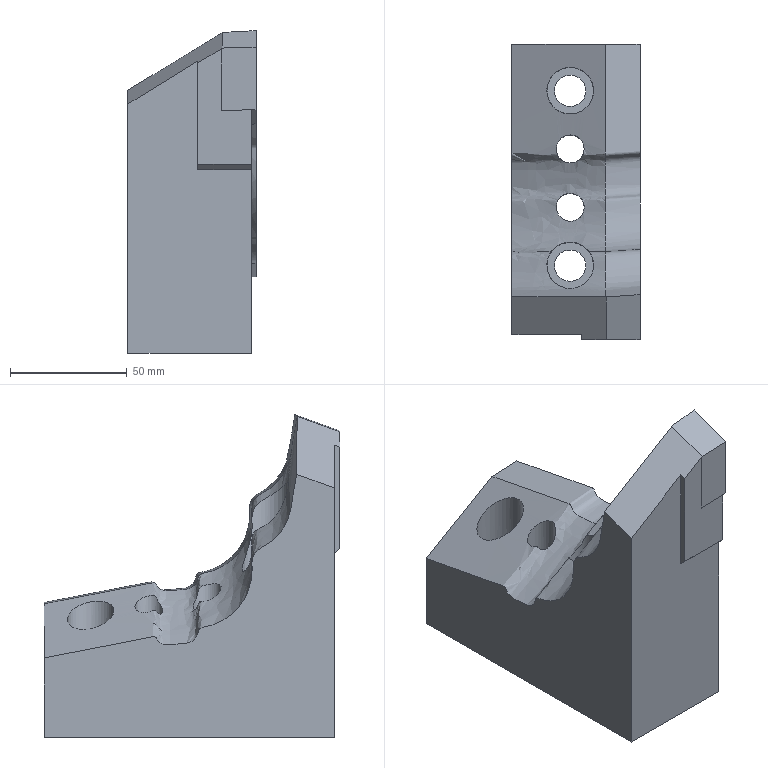Part | NX | features solid 2 | 1 solid | 25 faces | box 55 x 127 x 138.501 mm | volume 447238 mm3 | plane 11 | spline 8 | cylinder 6 | commonest cylinder face diameters 12 x2 13.5 x2 20 x2